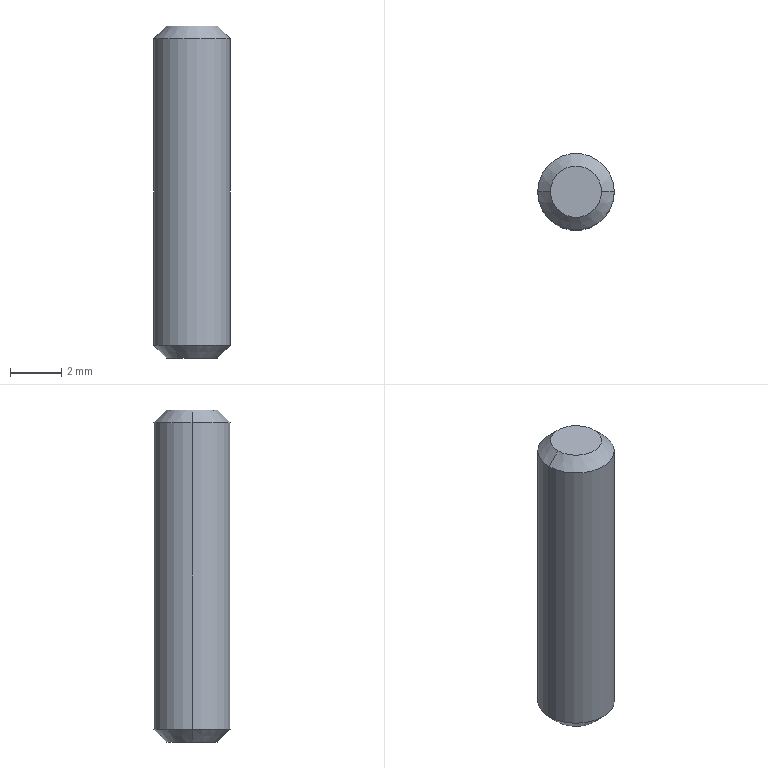Part | SolidWorks | features Chamfer 1, Extrusion 1 | 1 solid | 8 faces | box 3 x 3 x 13 mm | volume 89.797 mm3 | cone 4 | cylinder 2 | plane 2 | commonest cylinder face diameters 3 x2
STEP:
#1=CARTESIAN_POINT('',(-186.609,197.479,-13.));
#2=VERTEX_POINT('',#1);
#3=CARTESIAN_POINT('',(-184.609,197.479,-13.));
#4=VERTEX_POINT('',#3);
#5=CARTESIAN_POINT('',(-185.609,197.479,-13.));
#6=DIRECTION('',(0.,0.,-1.));
#7=DIRECTION('',(0.,-1.,0.));
#8=AXIS2_PLACEMENT_3D('',#5,#6,#7);
#9=CIRCLE('',#8,1.);
#10=EDGE_CURVE('',#2,#4,#9,.T.);
#11=ORIENTED_EDGE('',*,*,#10,.F.);
#12=CARTESIAN_POINT('',(-187.109,197.479,-12.5));
#13=VERTEX_POINT('',#12);
#14=CARTESIAN_POINT('',(-186.609,197.479,-13.));
#15=DIRECTION('',(-0.7071,0.,0.7071));
#16=VECTOR('',#15,1000.);
#17=LINE('',#14,#16);
#18=EDGE_CURVE('',#2,#13,#17,.T.);
#19=ORIENTED_EDGE('',*,*,#18,.T.);
#20=CARTESIAN_POINT('',(-184.109,197.479,-12.5));
#21=VERTEX_POINT('',#20);
#22=CARTESIAN_POINT('',(-185.609,197.479,-12.5));
#23=DIRECTION('',(0.,0.,1.));
#24=DIRECTION('',(1.,0.,0.));
#25=AXIS2_PLACEMENT_3D('',#22,#23,#24);
#26=CIRCLE('',#25,1.5);
#27=EDGE_CURVE('',#21,#13,#26,.T.);
#28=ORIENTED_EDGE('',*,*,#27,.F.);
#29=CARTESIAN_POINT('',(-184.609,197.479,-13.));
#30=DIRECTION('',(0.7071,0.,0.7071));
#31=VECTOR('',#30,1000.);
#32=LINE('',#29,#31);
#33=EDGE_CURVE('',#4,#21,#32,.T.);
#34=ORIENTED_EDGE('',*,*,#33,.F.);
#35=EDGE_LOOP('',(#11,#19,#28,#34));
#36=FACE_OUTER_BOUND('',#35,.T.);
#37=CARTESIAN_POINT('',(-185.609,197.479,-13.));
#38=DIRECTION('',(0.,0.,1.));
#39=DIRECTION('',(1.,0.,0.));
#40=AXIS2_PLACEMENT_3D('',#37,#38,#39);
#41=CONICAL_SURFACE('',#40,1.,0.7854);
#42=ADVANCED_FACE('',(#36),#41,.T.);
#43=CARTESIAN_POINT('',(-184.609,197.479,0.));
#44=VERTEX_POINT('',#43);
#45=CARTESIAN_POINT('',(-186.609,197.479,0.));
#46=VERTEX_POINT('',#45);
#47=CARTESIAN_POINT('',(-185.609,197.479,0.));
#48=DIRECTION('',(0.,0.,1.));
#49=DIRECTION('',(1.,0.,0.));
#50=AXIS2_PLACEMENT_3D('',#47,#48,#49);
#51=CIRCLE('',#50,1.);
#52=EDGE_CURVE('',#44,#46,#51,.T.);
#53=ORIENTED_EDGE('',*,*,#52,.F.);
#54=CARTESIAN_POINT('',(-184.109,197.479,-0.5));
#55=VERTEX_POINT('',#54);
#56=CARTESIAN_POINT('',(-184.609,197.479,0.));
#57=DIRECTION('',(0.7071,0.,-0.7071));
#58=VECTOR('',#57,1000.);
#59=LINE('',#56,#58);
#60=EDGE_CURVE('',#44,#55,#59,.T.);
#61=ORIENTED_EDGE('',*,*,#60,.T.);
#62=CARTESIAN_POINT('',(-187.109,197.479,-0.5));
#63=VERTEX_POINT('',#62);
#64=CARTESIAN_POINT('',(-185.609,197.479,-0.5));
#65=DIRECTION('',(0.,0.,-1.));
#66=DIRECTION('',(1.,0.,0.));
#67=AXIS2_PLACEMENT_3D('',#64,#65,#66);
#68=CIRCLE('',#67,1.5);
#69=EDGE_CURVE('',#63,#55,#68,.T.);
#70=ORIENTED_EDGE('',*,*,#69,.F.);
#71=CARTESIAN_POINT('',(-186.609,197.479,0.));
#72=DIRECTION('',(-0.7071,0.,-0.7071));
#73=VECTOR('',#72,1000.);
#74=LINE('',#71,#73);
#75=EDGE_CURVE('',#46,#63,#74,.T.);
#76=ORIENTED_EDGE('',*,*,#75,.F.);
#77=EDGE_LOOP('',(#53,#61,#70,#76));
#78=FACE_OUTER_BOUND('',#77,.T.);
#79=CARTESIAN_POINT('',(-185.609,197.479,0.));
#80=DIRECTION('',(0.,0.,-1.));
#81=DIRECTION('',(-1.,0.,0.));
#82=AXIS2_PLACEMENT_3D('',#79,#80,#81);
#83=CONICAL_SURFACE('',#82,1.,0.7854);
#84=ADVANCED_FACE('',(#78),#83,.T.);
#85=ORIENTED_EDGE('',*,*,#27,.T.);
#86=CARTESIAN_POINT('',(-187.109,197.479,-17.243));
#87=DIRECTION('',(0.,0.,1.));
#88=VECTOR('',#87,1000.);
#89=LINE('',#86,#88);
#90=EDGE_CURVE('',#13,#63,#89,.T.);
#91=ORIENTED_EDGE('',*,*,#90,.T.);
#92=ORIENTED_EDGE('',*,*,#69,.T.);
#93=CARTESIAN_POINT('',(-184.109,197.479,-17.243));
#94=DIRECTION('',(0.,0.,1.));
#95=VECTOR('',#94,1000.);
#96=LINE('',#93,#95);
#97=EDGE_CURVE('',#21,#55,#96,.T.);
#98=ORIENTED_EDGE('',*,*,#97,.F.);
#99=EDGE_LOOP('',(#85,#91,#92,#98));
#100=FACE_OUTER_BOUND('',#99,.T.);
#101=CARTESIAN_POINT('',(-185.609,197.479,-17.243));
#102=DIRECTION('',(0.,0.,1.));
#103=DIRECTION('',(1.,0.,0.));
#104=AXIS2_PLACEMENT_3D('',#101,#102,#103);
#105=CYLINDRICAL_SURFACE('',#104,1.5);
#106=ADVANCED_FACE('',(#100),#105,.T.);
#107=ORIENTED_EDGE('',*,*,#90,.F.);
#108=CARTESIAN_POINT('',(-185.609,197.479,-12.5));
#109=DIRECTION('',(0.,0.,1.));
#110=DIRECTION('',(1.,0.,0.));
#111=AXIS2_PLACEMENT_3D('',#108,#109,#110);
#112=CIRCLE('',#111,1.5);
#113=EDGE_CURVE('',#13,#21,#112,.T.);
#114=ORIENTED_EDGE('',*,*,#113,.T.);
#115=ORIENTED_EDGE('',*,*,#97,.T.);
#116=CARTESIAN_POINT('',(-185.609,197.479,-0.5));
#117=DIRECTION('',(0.,0.,-1.));
#118=DIRECTION('',(1.,0.,0.));
#119=AXIS2_PLACEMENT_3D('',#116,#117,#118);
#120=CIRCLE('',#119,1.5);
#121=EDGE_CURVE('',#55,#63,#120,.T.);
#122=ORIENTED_EDGE('',*,*,#121,.T.);
#123=EDGE_LOOP('',(#107,#114,#115,#122));
#124=FACE_OUTER_BOUND('',#123,.T.);
#125=CARTESIAN_POINT('',(-185.609,197.479,-17.243));
#126=DIRECTION('',(0.,0.,1.));
#127=DIRECTION('',(1.,0.,0.));
#128=AXIS2_PLACEMENT_3D('',#125,#126,#127);
#129=CYLINDRICAL_SURFACE('',#128,1.5);
#130=ADVANCED_FACE('',(#124),#129,.T.);
#131=CARTESIAN_POINT('',(-185.609,197.479,0.));
#132=DIRECTION('',(0.,0.,1.));
#133=DIRECTION('',(1.,0.,0.));
#134=AXIS2_PLACEMENT_3D('',#131,#132,#133);
#135=CIRCLE('',#134,1.);
#136=EDGE_CURVE('',#46,#44,#135,.T.);
#137=ORIENTED_EDGE('',*,*,#136,.T.);
#138=ORIENTED_EDGE('',*,*,#52,.T.);
#139=EDGE_LOOP('',(#137,#138));
#140=FACE_OUTER_BOUND('',#139,.T.);
#141=CARTESIAN_POINT('',(-185.609,197.479,0.));
#142=DIRECTION('',(0.,0.,1.));
#143=DIRECTION('',(1.,0.,0.));
#144=AXIS2_PLACEMENT_3D('',#141,#142,#143);
#145=PLANE('',#144);
#146=ADVANCED_FACE('',(#140),#145,.T.);
#147=CARTESIAN_POINT('',(-185.609,197.479,-13.));
#148=DIRECTION('',(0.,0.,-1.));
#149=DIRECTION('',(0.,-1.,0.));
#150=AXIS2_PLACEMENT_3D('',#147,#148,#149);
#151=CIRCLE('',#150,1.);
#152=EDGE_CURVE('',#4,#2,#151,.T.);
#153=ORIENTED_EDGE('',*,*,#152,.T.);
#154=ORIENTED_EDGE('',*,*,#10,.T.);
#155=EDGE_LOOP('',(#153,#154));
#156=FACE_OUTER_BOUND('',#155,.T.);
#157=CARTESIAN_POINT('',(-441.963,151.38,-13.));
#158=DIRECTION('',(0.,0.,1.));
#159=DIRECTION('',(0.79,-0.6131,0.));
#160=AXIS2_PLACEMENT_3D('',#157,#158,#159);
#161=PLANE('',#160);
#162=ADVANCED_FACE('',(#156),#161,.F.);
#163=ORIENTED_EDGE('',*,*,#60,.F.);
#164=ORIENTED_EDGE('',*,*,#136,.F.);
#165=ORIENTED_EDGE('',*,*,#75,.T.);
#166=ORIENTED_EDGE('',*,*,#121,.F.);
#167=EDGE_LOOP('',(#163,#164,#165,#166));
#168=FACE_OUTER_BOUND('',#167,.T.);
#169=CARTESIAN_POINT('',(-185.609,197.479,0.));
#170=DIRECTION('',(0.,0.,-1.));
#171=DIRECTION('',(-1.,0.,0.));
#172=AXIS2_PLACEMENT_3D('',#169,#170,#171);
#173=CONICAL_SURFACE('',#172,1.,0.7854);
#174=ADVANCED_FACE('',(#168),#173,.T.);
#175=ORIENTED_EDGE('',*,*,#18,.F.);
#176=ORIENTED_EDGE('',*,*,#152,.F.);
#177=ORIENTED_EDGE('',*,*,#33,.T.);
#178=ORIENTED_EDGE('',*,*,#113,.F.);
#179=EDGE_LOOP('',(#175,#176,#177,#178));
#180=FACE_OUTER_BOUND('',#179,.T.);
#181=CARTESIAN_POINT('',(-185.609,197.479,-13.));
#182=DIRECTION('',(0.,0.,1.));
#183=DIRECTION('',(1.,0.,0.));
#184=AXIS2_PLACEMENT_3D('',#181,#182,#183);
#185=CONICAL_SURFACE('',#184,1.,0.7854);
#186=ADVANCED_FACE('',(#180),#185,.T.);
#187=CLOSED_SHELL('',(#42,#84,#106,#130,#146,#162,#174,#186));
#188=MANIFOLD_SOLID_BREP('',#187);
#189=CARTESIAN_POINT('',(0.,0.,0.));
#190=DIRECTION('',(0.,0.,1.));
#191=DIRECTION('',(1.,0.,0.));
#192=AXIS2_PLACEMENT_3D('',#189,#190,#191);
#193=(LENGTH_UNIT()NAMED_UNIT(*)SI_UNIT(.MILLI.,.METRE.));
#194=UNCERTAINTY_MEASURE_WITH_UNIT(LENGTH_MEASURE(0.00001),#193,'','');
#195=(NAMED_UNIT(*)PLANE_ANGLE_UNIT()SI_UNIT($,.RADIAN.));
#196=(NAMED_UNIT(*)SI_UNIT($,.STERADIAN.)SOLID_ANGLE_UNIT());
#197=(GEOMETRIC_REPRESENTATION_CONTEXT(3)GLOBAL_UNCERTAINTY_ASSIGNED_CONTEXT((#194))GLOBAL_UNIT_ASSIGNED_CONTEXT((#193,#195,#196))REPRESENTATION_CONTEXT('',''));
#198=ADVANCED_BREP_SHAPE_REPRESENTATION('',(#188,#192),#197);